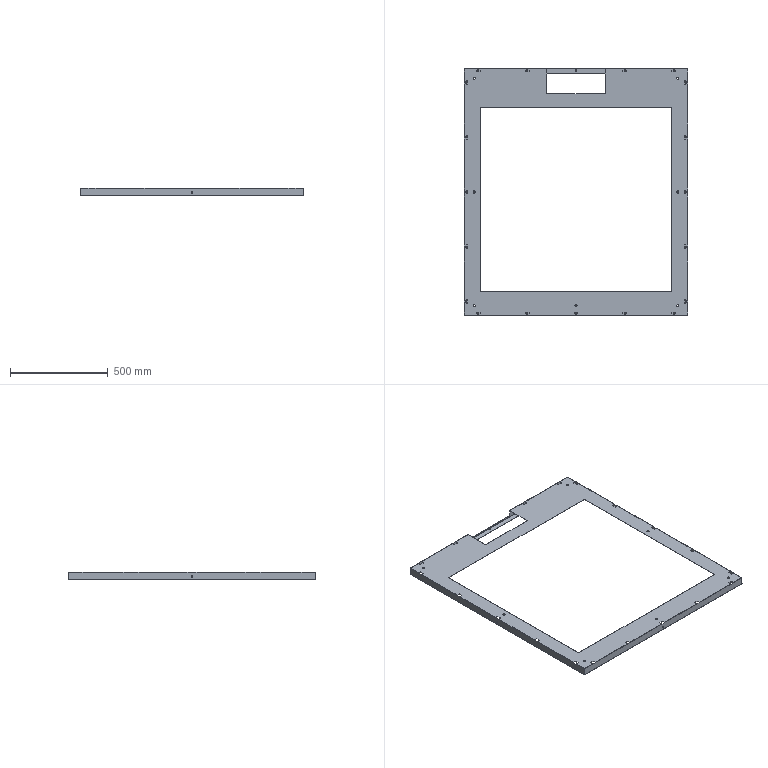Part | SolidWorks | features ICE 8, EdgeFlange 2, FlatPattern 1, SMBaseFlange 1, SheetMetal 1 | 1 solid | 384 faces | box 1139 x 1259 x 40 mm | volume 764574 mm3 | plane 242 | cylinder 126 | spline 16 | commonest cylinder face diameters 7 x50 0.4 x28 2.4 x28 11 x14 10 x6